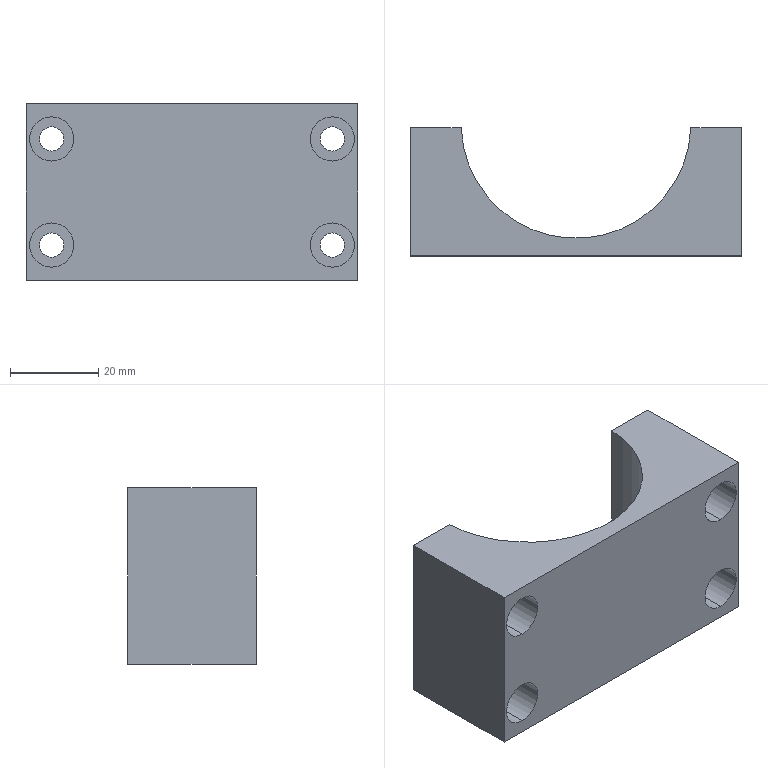Part | SolidWorks | features Extrusion 1, HoleWzd 1, ICE 1, MoveFace 1 | 1 solid | 28 faces | box 75 x 29 x 40 mm | volume 38371 mm3 | cylinder 17 | plane 11 | commonest cylinder face diameters 5.5 x8 10 x8 52 x1
STEP:
#1=CARTESIAN_POINT('',(-31.75,10.,13.));
#2=VERTEX_POINT('',#1);
#3=CARTESIAN_POINT('',(-31.75,10.,3.));
#4=VERTEX_POINT('',#3);
#5=CARTESIAN_POINT('',(-31.75,10.,8.));
#6=DIRECTION('',(0.,-1.,0.));
#7=DIRECTION('',(0.,0.,-1.));
#8=AXIS2_PLACEMENT_3D('',#5,#6,#7);
#9=CIRCLE('',#8,5.);
#10=EDGE_CURVE('',#2,#4,#9,.T.);
#11=ORIENTED_EDGE('',*,*,#10,.F.);
#12=CARTESIAN_POINT('',(-31.75,-15.,13.));
#13=VERTEX_POINT('',#12);
#14=CARTESIAN_POINT('',(-31.75,-15.,13.));
#15=DIRECTION('',(0.,-1.,0.));
#16=VECTOR('',#15,1000.);
#17=LINE('',#14,#16);
#18=EDGE_CURVE('',#2,#13,#17,.T.);
#19=ORIENTED_EDGE('',*,*,#18,.T.);
#20=CARTESIAN_POINT('',(-31.75,-15.,3.));
#21=VERTEX_POINT('',#20);
#22=CARTESIAN_POINT('',(-31.75,-15.,8.));
#23=DIRECTION('',(0.,-1.,0.));
#24=DIRECTION('',(0.,0.,-1.));
#25=AXIS2_PLACEMENT_3D('',#22,#23,#24);
#26=CIRCLE('',#25,5.);
#27=EDGE_CURVE('',#13,#21,#26,.T.);
#28=ORIENTED_EDGE('',*,*,#27,.T.);
#29=CARTESIAN_POINT('',(-31.75,-15.,3.));
#30=DIRECTION('',(0.,-1.,0.));
#31=VECTOR('',#30,1000.);
#32=LINE('',#29,#31);
#33=EDGE_CURVE('',#4,#21,#32,.T.);
#34=ORIENTED_EDGE('',*,*,#33,.F.);
#35=EDGE_LOOP('',(#11,#19,#28,#34));
#36=FACE_OUTER_BOUND('',#35,.T.);
#37=CARTESIAN_POINT('',(-31.75,-15.,8.));
#38=DIRECTION('',(0.,-1.,0.));
#39=DIRECTION('',(0.,0.,-1.));
#40=AXIS2_PLACEMENT_3D('',#37,#38,#39);
#41=CYLINDRICAL_SURFACE('',#40,5.);
#42=ADVANCED_FACE('',(#36),#41,.F.);
#43=CARTESIAN_POINT('',(-31.75,14.,10.75));
#44=VERTEX_POINT('',#43);
#45=CARTESIAN_POINT('',(-31.75,14.,5.25));
#46=VERTEX_POINT('',#45);
#47=CARTESIAN_POINT('',(-31.75,14.,8.));
#48=DIRECTION('',(0.,-1.,0.));
#49=DIRECTION('',(0.,0.,-1.));
#50=AXIS2_PLACEMENT_3D('',#47,#48,#49);
#51=CIRCLE('',#50,2.75);
#52=EDGE_CURVE('',#44,#46,#51,.T.);
#53=ORIENTED_EDGE('',*,*,#52,.F.);
#54=CARTESIAN_POINT('',(-31.75,10.,10.75));
#55=VERTEX_POINT('',#54);
#56=CARTESIAN_POINT('',(-31.75,-15.,10.75));
#57=DIRECTION('',(0.,-1.,0.));
#58=VECTOR('',#57,1000.);
#59=LINE('',#56,#58);
#60=EDGE_CURVE('',#44,#55,#59,.T.);
#61=ORIENTED_EDGE('',*,*,#60,.T.);
#62=CARTESIAN_POINT('',(-31.75,10.,5.25));
#63=VERTEX_POINT('',#62);
#64=CARTESIAN_POINT('',(-31.75,10.,8.));
#65=DIRECTION('',(0.,-1.,0.));
#66=DIRECTION('',(0.,0.,-1.));
#67=AXIS2_PLACEMENT_3D('',#64,#65,#66);
#68=CIRCLE('',#67,2.75);
#69=EDGE_CURVE('',#55,#63,#68,.T.);
#70=ORIENTED_EDGE('',*,*,#69,.T.);
#71=CARTESIAN_POINT('',(-31.75,-15.,5.25));
#72=DIRECTION('',(0.,-1.,0.));
#73=VECTOR('',#72,1000.);
#74=LINE('',#71,#73);
#75=EDGE_CURVE('',#46,#63,#74,.T.);
#76=ORIENTED_EDGE('',*,*,#75,.F.);
#77=EDGE_LOOP('',(#53,#61,#70,#76));
#78=FACE_OUTER_BOUND('',#77,.T.);
#79=CARTESIAN_POINT('',(-31.75,-15.,8.));
#80=DIRECTION('',(0.,-1.,0.));
#81=DIRECTION('',(0.,0.,-1.));
#82=AXIS2_PLACEMENT_3D('',#79,#80,#81);
#83=CYLINDRICAL_SURFACE('',#82,2.75);
#84=ADVANCED_FACE('',(#78),#83,.F.);
#85=CARTESIAN_POINT('',(-31.75,10.,37.));
#86=VERTEX_POINT('',#85);
#87=CARTESIAN_POINT('',(-31.75,10.,27.));
#88=VERTEX_POINT('',#87);
#89=CARTESIAN_POINT('',(-31.75,10.,32.));
#90=DIRECTION('',(0.,-1.,0.));
#91=DIRECTION('',(0.,0.,-1.));
#92=AXIS2_PLACEMENT_3D('',#89,#90,#91);
#93=CIRCLE('',#92,5.);
#94=EDGE_CURVE('',#86,#88,#93,.T.);
#95=ORIENTED_EDGE('',*,*,#94,.F.);
#96=CARTESIAN_POINT('',(-31.75,-15.,37.));
#97=VERTEX_POINT('',#96);
#98=CARTESIAN_POINT('',(-31.75,-15.,37.));
#99=DIRECTION('',(0.,-1.,0.));
#100=VECTOR('',#99,1000.);
#101=LINE('',#98,#100);
#102=EDGE_CURVE('',#86,#97,#101,.T.);
#103=ORIENTED_EDGE('',*,*,#102,.T.);
#104=CARTESIAN_POINT('',(-31.75,-15.,27.));
#105=VERTEX_POINT('',#104);
#106=CARTESIAN_POINT('',(-31.75,-15.,32.));
#107=DIRECTION('',(0.,-1.,0.));
#108=DIRECTION('',(0.,0.,-1.));
#109=AXIS2_PLACEMENT_3D('',#106,#107,#108);
#110=CIRCLE('',#109,5.);
#111=EDGE_CURVE('',#97,#105,#110,.T.);
#112=ORIENTED_EDGE('',*,*,#111,.T.);
#113=CARTESIAN_POINT('',(-31.75,-15.,27.));
#114=DIRECTION('',(0.,-1.,0.));
#115=VECTOR('',#114,1000.);
#116=LINE('',#113,#115);
#117=EDGE_CURVE('',#88,#105,#116,.T.);
#118=ORIENTED_EDGE('',*,*,#117,.F.);
#119=EDGE_LOOP('',(#95,#103,#112,#118));
#120=FACE_OUTER_BOUND('',#119,.T.);
#121=CARTESIAN_POINT('',(-31.75,-15.,32.));
#122=DIRECTION('',(0.,-1.,0.));
#123=DIRECTION('',(0.,0.,-1.));
#124=AXIS2_PLACEMENT_3D('',#121,#122,#123);
#125=CYLINDRICAL_SURFACE('',#124,5.);
#126=ADVANCED_FACE('',(#120),#125,.F.);
#127=CARTESIAN_POINT('',(-31.75,14.,34.75));
#128=VERTEX_POINT('',#127);
#129=CARTESIAN_POINT('',(-31.75,14.,29.25));
#130=VERTEX_POINT('',#129);
#131=CARTESIAN_POINT('',(-31.75,14.,32.));
#132=DIRECTION('',(0.,-1.,0.));
#133=DIRECTION('',(0.,0.,-1.));
#134=AXIS2_PLACEMENT_3D('',#131,#132,#133);
#135=CIRCLE('',#134,2.75);
#136=EDGE_CURVE('',#128,#130,#135,.T.);
#137=ORIENTED_EDGE('',*,*,#136,.F.);
#138=CARTESIAN_POINT('',(-31.75,10.,34.75));
#139=VERTEX_POINT('',#138);
#140=CARTESIAN_POINT('',(-31.75,-15.,34.75));
#141=DIRECTION('',(0.,-1.,0.));
#142=VECTOR('',#141,1000.);
#143=LINE('',#140,#142);
#144=EDGE_CURVE('',#128,#139,#143,.T.);
#145=ORIENTED_EDGE('',*,*,#144,.T.);
#146=CARTESIAN_POINT('',(-31.75,10.,29.25));
#147=VERTEX_POINT('',#146);
#148=CARTESIAN_POINT('',(-31.75,10.,32.));
#149=DIRECTION('',(0.,-1.,0.));
#150=DIRECTION('',(0.,0.,-1.));
#151=AXIS2_PLACEMENT_3D('',#148,#149,#150);
#152=CIRCLE('',#151,2.75);
#153=EDGE_CURVE('',#139,#147,#152,.T.);
#154=ORIENTED_EDGE('',*,*,#153,.T.);
#155=CARTESIAN_POINT('',(-31.75,-15.,29.25));
#156=DIRECTION('',(0.,-1.,0.));
#157=VECTOR('',#156,1000.);
#158=LINE('',#155,#157);
#159=EDGE_CURVE('',#130,#147,#158,.T.);
#160=ORIENTED_EDGE('',*,*,#159,.F.);
#161=EDGE_LOOP('',(#137,#145,#154,#160));
#162=FACE_OUTER_BOUND('',#161,.T.);
#163=CARTESIAN_POINT('',(-31.75,-15.,32.));
#164=DIRECTION('',(0.,-1.,0.));
#165=DIRECTION('',(0.,0.,-1.));
#166=AXIS2_PLACEMENT_3D('',#163,#164,#165);
#167=CYLINDRICAL_SURFACE('',#166,2.75);
#168=ADVANCED_FACE('',(#162),#167,.F.);
#169=CARTESIAN_POINT('',(31.75,10.,37.));
#170=VERTEX_POINT('',#169);
#171=CARTESIAN_POINT('',(31.75,10.,27.));
#172=VERTEX_POINT('',#171);
#173=CARTESIAN_POINT('',(31.75,10.,32.));
#174=DIRECTION('',(0.,-1.,0.));
#175=DIRECTION('',(0.,0.,-1.));
#176=AXIS2_PLACEMENT_3D('',#173,#174,#175);
#177=CIRCLE('',#176,5.);
#178=EDGE_CURVE('',#170,#172,#177,.T.);
#179=ORIENTED_EDGE('',*,*,#178,.F.);
#180=CARTESIAN_POINT('',(31.75,-15.,37.));
#181=VERTEX_POINT('',#180);
#182=CARTESIAN_POINT('',(31.75,-15.,37.));
#183=DIRECTION('',(0.,-1.,0.));
#184=VECTOR('',#183,1000.);
#185=LINE('',#182,#184);
#186=EDGE_CURVE('',#170,#181,#185,.T.);
#187=ORIENTED_EDGE('',*,*,#186,.T.);
#188=CARTESIAN_POINT('',(31.75,-15.,27.));
#189=VERTEX_POINT('',#188);
#190=CARTESIAN_POINT('',(31.75,-15.,32.));
#191=DIRECTION('',(0.,-1.,0.));
#192=DIRECTION('',(0.,0.,-1.));
#193=AXIS2_PLACEMENT_3D('',#190,#191,#192);
#194=CIRCLE('',#193,5.);
#195=EDGE_CURVE('',#181,#189,#194,.T.);
#196=ORIENTED_EDGE('',*,*,#195,.T.);
#197=CARTESIAN_POINT('',(31.75,-15.,27.));
#198=DIRECTION('',(0.,-1.,0.));
#199=VECTOR('',#198,1000.);
#200=LINE('',#197,#199);
#201=EDGE_CURVE('',#172,#189,#200,.T.);
#202=ORIENTED_EDGE('',*,*,#201,.F.);
#203=EDGE_LOOP('',(#179,#187,#196,#202));
#204=FACE_OUTER_BOUND('',#203,.T.);
#205=CARTESIAN_POINT('',(31.75,-15.,32.));
#206=DIRECTION('',(0.,-1.,0.));
#207=DIRECTION('',(0.,0.,-1.));
#208=AXIS2_PLACEMENT_3D('',#205,#206,#207);
#209=CYLINDRICAL_SURFACE('',#208,5.);
#210=ADVANCED_FACE('',(#204),#209,.F.);
#211=CARTESIAN_POINT('',(31.75,14.,34.75));
#212=VERTEX_POINT('',#211);
#213=CARTESIAN_POINT('',(31.75,14.,29.25));
#214=VERTEX_POINT('',#213);
#215=CARTESIAN_POINT('',(31.75,14.,32.));
#216=DIRECTION('',(0.,-1.,0.));
#217=DIRECTION('',(0.,0.,-1.));
#218=AXIS2_PLACEMENT_3D('',#215,#216,#217);
#219=CIRCLE('',#218,2.75);
#220=EDGE_CURVE('',#212,#214,#219,.T.);
#221=ORIENTED_EDGE('',*,*,#220,.F.);
#222=CARTESIAN_POINT('',(31.75,10.,34.75));
#223=VERTEX_POINT('',#222);
#224=CARTESIAN_POINT('',(31.75,-15.,34.75));
#225=DIRECTION('',(0.,-1.,0.));
#226=VECTOR('',#225,1000.);
#227=LINE('',#224,#226);
#228=EDGE_CURVE('',#212,#223,#227,.T.);
#229=ORIENTED_EDGE('',*,*,#228,.T.);
#230=CARTESIAN_POINT('',(31.75,10.,29.25));
#231=VERTEX_POINT('',#230);
#232=CARTESIAN_POINT('',(31.75,10.,32.));
#233=DIRECTION('',(0.,-1.,0.));
#234=DIRECTION('',(0.,0.,-1.));
#235=AXIS2_PLACEMENT_3D('',#232,#233,#234);
#236=CIRCLE('',#235,2.75);
#237=EDGE_CURVE('',#223,#231,#236,.T.);
#238=ORIENTED_EDGE('',*,*,#237,.T.);
#239=CARTESIAN_POINT('',(31.75,-15.,29.25));
#240=DIRECTION('',(0.,-1.,0.));
#241=VECTOR('',#240,1000.);
#242=LINE('',#239,#241);
#243=EDGE_CURVE('',#214,#231,#242,.T.);
#244=ORIENTED_EDGE('',*,*,#243,.F.);
#245=EDGE_LOOP('',(#221,#229,#238,#244));
#246=FACE_OUTER_BOUND('',#245,.T.);
#247=CARTESIAN_POINT('',(31.75,-15.,32.));
#248=DIRECTION('',(0.,-1.,0.));
#249=DIRECTION('',(0.,0.,-1.));
#250=AXIS2_PLACEMENT_3D('',#247,#248,#249);
#251=CYLINDRICAL_SURFACE('',#250,2.75);
#252=ADVANCED_FACE('',(#246),#251,.F.);
#253=CARTESIAN_POINT('',(31.75,10.,13.));
#254=VERTEX_POINT('',#253);
#255=CARTESIAN_POINT('',(31.75,10.,3.));
#256=VERTEX_POINT('',#255);
#257=CARTESIAN_POINT('',(31.75,10.,8.));
#258=DIRECTION('',(0.,-1.,0.));
#259=DIRECTION('',(0.,0.,-1.));
#260=AXIS2_PLACEMENT_3D('',#257,#258,#259);
#261=CIRCLE('',#260,5.);
#262=EDGE_CURVE('',#254,#256,#261,.T.);
#263=ORIENTED_EDGE('',*,*,#262,.F.);
#264=CARTESIAN_POINT('',(31.75,-15.,13.));
#265=VERTEX_POINT('',#264);
#266=CARTESIAN_POINT('',(31.75,-15.,13.));
#267=DIRECTION('',(0.,-1.,0.));
#268=VECTOR('',#267,1000.);
#269=LINE('',#266,#268);
#270=EDGE_CURVE('',#254,#265,#269,.T.);
#271=ORIENTED_EDGE('',*,*,#270,.T.);
#272=CARTESIAN_POINT('',(31.75,-15.,3.));
#273=VERTEX_POINT('',#272);
#274=CARTESIAN_POINT('',(31.75,-15.,8.));
#275=DIRECTION('',(0.,-1.,0.));
#276=DIRECTION('',(0.,0.,-1.));
#277=AXIS2_PLACEMENT_3D('',#274,#275,#276);
#278=CIRCLE('',#277,5.);
#279=EDGE_CURVE('',#265,#273,#278,.T.);
#280=ORIENTED_EDGE('',*,*,#279,.T.);
#281=CARTESIAN_POINT('',(31.75,-15.,3.));
#282=DIRECTION('',(0.,-1.,0.));
#283=VECTOR('',#282,1000.);
#284=LINE('',#281,#283);
#285=EDGE_CURVE('',#256,#273,#284,.T.);
#286=ORIENTED_EDGE('',*,*,#285,.F.);
#287=EDGE_LOOP('',(#263,#271,#280,#286));
#288=FACE_OUTER_BOUND('',#287,.T.);
#289=CARTESIAN_POINT('',(31.75,-15.,8.));
#290=DIRECTION('',(0.,-1.,0.));
#291=DIRECTION('',(0.,0.,-1.));
#292=AXIS2_PLACEMENT_3D('',#289,#290,#291);
#293=CYLINDRICAL_SURFACE('',#292,5.);
#294=ADVANCED_FACE('',(#288),#293,.F.);
#295=CARTESIAN_POINT('',(31.75,14.,10.75));
#296=VERTEX_POINT('',#295);
#297=CARTESIAN_POINT('',(31.75,14.,5.25));
#298=VERTEX_POINT('',#297);
#299=CARTESIAN_POINT('',(31.75,14.,8.));
#300=DIRECTION('',(0.,-1.,0.));
#301=DIRECTION('',(0.,0.,-1.));
#302=AXIS2_PLACEMENT_3D('',#299,#300,#301);
#303=CIRCLE('',#302,2.75);
#304=EDGE_CURVE('',#296,#298,#303,.T.);
#305=ORIENTED_EDGE('',*,*,#304,.F.);
#306=CARTESIAN_POINT('',(31.75,10.,10.75));
#307=VERTEX_POINT('',#306);
#308=CARTESIAN_POINT('',(31.75,-15.,10.75));
#309=DIRECTION('',(0.,-1.,0.));
#310=VECTOR('',#309,1000.);
#311=LINE('',#308,#310);
#312=EDGE_CURVE('',#296,#307,#311,.T.);
#313=ORIENTED_EDGE('',*,*,#312,.T.);
#314=CARTESIAN_POINT('',(31.75,10.,5.25));
#315=VERTEX_POINT('',#314);
#316=CARTESIAN_POINT('',(31.75,10.,8.));
#317=DIRECTION('',(0.,-1.,0.));
#318=DIRECTION('',(0.,0.,-1.));
#319=AXIS2_PLACEMENT_3D('',#316,#317,#318);
#320=CIRCLE('',#319,2.75);
#321=EDGE_CURVE('',#307,#315,#320,.T.);
#322=ORIENTED_EDGE('',*,*,#321,.T.);
#323=CARTESIAN_POINT('',(31.75,-15.,5.25));
#324=DIRECTION('',(0.,-1.,0.));
#325=VECTOR('',#324,1000.);
#326=LINE('',#323,#325);
#327=EDGE_CURVE('',#298,#315,#326,.T.);
#328=ORIENTED_EDGE('',*,*,#327,.F.);
#329=EDGE_LOOP('',(#305,#313,#322,#328));
#330=FACE_OUTER_BOUND('',#329,.T.);
#331=CARTESIAN_POINT('',(31.75,-15.,8.));
#332=DIRECTION('',(0.,-1.,0.));
#333=DIRECTION('',(0.,0.,-1.));
#334=AXIS2_PLACEMENT_3D('',#331,#332,#333);
#335=CYLINDRICAL_SURFACE('',#334,2.75);
#336=ADVANCED_FACE('',(#330),#335,.F.);
#337=CARTESIAN_POINT('',(31.75,14.,32.));
#338=DIRECTION('',(0.,-1.,0.));
#339=DIRECTION('',(0.,0.,-1.));
#340=AXIS2_PLACEMENT_3D('',#337,#338,#339);
#341=CIRCLE('',#340,2.75);
#342=EDGE_CURVE('',#214,#212,#341,.T.);
#343=ORIENTED_EDGE('',*,*,#342,.T.);
#344=ORIENTED_EDGE('',*,*,#220,.T.);
#345=EDGE_LOOP('',(#343,#344));
#346=FACE_BOUND('',#345,.T.);
#347=CARTESIAN_POINT('',(31.75,14.,8.));
#348=DIRECTION('',(0.,-1.,0.));
#349=DIRECTION('',(0.,0.,-1.));
#350=AXIS2_PLACEMENT_3D('',#347,#348,#349);
#351=CIRCLE('',#350,2.75);
#352=EDGE_CURVE('',#298,#296,#351,.T.);
#353=ORIENTED_EDGE('',*,*,#352,.T.);
#354=ORIENTED_EDGE('',*,*,#304,.T.);
#355=EDGE_LOOP('',(#353,#354));
#356=FACE_BOUND('',#355,.T.);
#357=CARTESIAN_POINT('',(37.5,14.,0.));
#358=VERTEX_POINT('',#357);
#359=CARTESIAN_POINT('',(25.981,14.,0.));
#360=VERTEX_POINT('',#359);
#361=CARTESIAN_POINT('',(-37.5,14.,0.));
#362=DIRECTION('',(-1.,0.,0.));
#363=VECTOR('',#362,1000.);
#364=LINE('',#361,#363);
#365=EDGE_CURVE('',#358,#360,#364,.T.);
#366=ORIENTED_EDGE('',*,*,#365,.T.);
#367=CARTESIAN_POINT('',(25.981,14.,40.));
#368=VERTEX_POINT('',#367);
#369=CARTESIAN_POINT('',(25.981,14.,0.));
#370=DIRECTION('',(0.,0.,1.));
#371=VECTOR('',#370,1000.);
#372=LINE('',#369,#371);
#373=EDGE_CURVE('',#360,#368,#372,.T.);
#374=ORIENTED_EDGE('',*,*,#373,.T.);
#375=CARTESIAN_POINT('',(37.5,14.,40.));
#376=VERTEX_POINT('',#375);
#377=CARTESIAN_POINT('',(-37.5,14.,40.));
#378=DIRECTION('',(-1.,0.,0.));
#379=VECTOR('',#378,1000.);
#380=LINE('',#377,#379);
#381=EDGE_CURVE('',#376,#368,#380,.T.);
#382=ORIENTED_EDGE('',*,*,#381,.F.);
#383=CARTESIAN_POINT('',(37.5,14.,40.));
#384=DIRECTION('',(0.,0.,-1.));
#385=VECTOR('',#384,1000.);
#386=LINE('',#383,#385);
#387=EDGE_CURVE('',#376,#358,#386,.T.);
#388=ORIENTED_EDGE('',*,*,#387,.T.);
#389=EDGE_LOOP('',(#366,#374,#382,#388));
#390=FACE_OUTER_BOUND('',#389,.T.);
#391=CARTESIAN_POINT('',(-37.5,14.,40.));
#392=DIRECTION('',(0.,-1.,0.));
#393=DIRECTION('',(0.,0.,-1.));
#394=AXIS2_PLACEMENT_3D('',#391,#392,#393);
#395=PLANE('',#394);
#396=ADVANCED_FACE('',(#346,#356,#390),#395,.F.);
#397=CARTESIAN_POINT('',(37.5,-15.,0.));
#398=VERTEX_POINT('',#397);
#399=CARTESIAN_POINT('',(37.5,-15.,0.));
#400=DIRECTION('',(0.,1.,0.));
#401=VECTOR('',#400,1000.);
#402=LINE('',#399,#401);
#403=EDGE_CURVE('',#398,#358,#402,.T.);
#404=ORIENTED_EDGE('',*,*,#403,.T.);
#405=ORIENTED_EDGE('',*,*,#387,.F.);
#406=CARTESIAN_POINT('',(37.5,-15.,40.));
#407=VERTEX_POINT('',#406);
#408=CARTESIAN_POINT('',(37.5,-15.,40.));
#409=DIRECTION('',(0.,1.,0.));
#410=VECTOR('',#409,1000.);
#411=LINE('',#408,#410);
#412=EDGE_CURVE('',#407,#376,#411,.T.);
#413=ORIENTED_EDGE('',*,*,#412,.F.);
#414=CARTESIAN_POINT('',(37.5,-15.,40.));
#415=DIRECTION('',(0.,0.,-1.));
#416=VECTOR('',#415,1000.);
#417=LINE('',#414,#416);
#418=EDGE_CURVE('',#407,#398,#417,.T.);
#419=ORIENTED_EDGE('',*,*,#418,.T.);
#420=EDGE_LOOP('',(#404,#405,#413,#419));
#421=FACE_OUTER_BOUND('',#420,.T.);
#422=CARTESIAN_POINT('',(37.5,-15.,40.));
#423=DIRECTION('',(-1.,0.,0.));
#424=DIRECTION('',(0.,0.,1.));
#425=AXIS2_PLACEMENT_3D('',#422,#423,#424);
#426=PLANE('',#425);
#427=ADVANCED_FACE('',(#421),#426,.F.);
#428=CARTESIAN_POINT('',(-31.75,14.,8.));
#429=DIRECTION('',(0.,-1.,0.));
#430=DIRECTION('',(0.,0.,-1.));
#431=AXIS2_PLACEMENT_3D('',#428,#429,#430);
#432=CIRCLE('',#431,2.75);
#433=EDGE_CURVE('',#46,#44,#432,.T.);
#434=ORIENTED_EDGE('',*,*,#433,.T.);
#435=ORIENTED_EDGE('',*,*,#52,.T.);
#436=EDGE_LOOP('',(#434,#435));
#437=FACE_BOUND('',#436,.T.);
#438=CARTESIAN_POINT('',(-31.75,14.,32.));
#439=DIRECTION('',(0.,-1.,0.));
#440=DIRECTION('',(0.,0.,-1.));
#441=AXIS2_PLACEMENT_3D('',#438,#439,#440);
#442=CIRCLE('',#441,2.75);
#443=EDGE_CURVE('',#130,#128,#442,.T.);
#444=ORIENTED_EDGE('',*,*,#443,.T.);
#445=ORIENTED_EDGE('',*,*,#136,.T.);
#446=EDGE_LOOP('',(#444,#445));
#447=FACE_BOUND('',#446,.T.);
#448=CARTESIAN_POINT('',(-25.981,14.,40.));
#449=VERTEX_POINT('',#448);
#450=CARTESIAN_POINT('',(-37.5,14.,40.));
#451=VERTEX_POINT('',#450);
#452=CARTESIAN_POINT('',(-37.5,14.,40.));
#453=DIRECTION('',(-1.,0.,0.));
#454=VECTOR('',#453,1000.);
#455=LINE('',#452,#454);
#456=EDGE_CURVE('',#449,#451,#455,.T.);
#457=ORIENTED_EDGE('',*,*,#456,.F.);
#458=CARTESIAN_POINT('',(-25.981,14.,0.));
#459=VERTEX_POINT('',#458);
#460=CARTESIAN_POINT('',(-25.981,14.,40.));
#461=DIRECTION('',(0.,0.,-1.));
#462=VECTOR('',#461,1000.);
#463=LINE('',#460,#462);
#464=EDGE_CURVE('',#449,#459,#463,.T.);
#465=ORIENTED_EDGE('',*,*,#464,.T.);
#466=CARTESIAN_POINT('',(-37.5,14.,0.));
#467=VERTEX_POINT('',#466);
#468=CARTESIAN_POINT('',(-37.5,14.,0.));
#469=DIRECTION('',(-1.,0.,0.));
#470=VECTOR('',#469,1000.);
#471=LINE('',#468,#470);
#472=EDGE_CURVE('',#459,#467,#471,.T.);
#473=ORIENTED_EDGE('',*,*,#472,.T.);
#474=CARTESIAN_POINT('',(-37.5,14.,40.));
#475=DIRECTION('',(0.,0.,-1.));
#476=VECTOR('',#475,1000.);
#477=LINE('',#474,#476);
#478=EDGE_CURVE('',#451,#467,#477,.T.);
#479=ORIENTED_EDGE('',*,*,#478,.F.);
#480=EDGE_LOOP('',(#457,#465,#473,#479));
#481=FACE_OUTER_BOUND('',#480,.T.);
#482=CARTESIAN_POINT('',(-37.5,14.,40.));
#483=DIRECTION('',(0.,-1.,0.));
#484=DIRECTION('',(0.,0.,-1.));
#485=AXIS2_PLACEMENT_3D('',#482,#483,#484);
#486=PLANE('',#485);
#487=ADVANCED_FACE('',(#437,#447,#481),#486,.F.);
#488=CARTESIAN_POINT('',(-37.5,-15.,0.));
#489=VERTEX_POINT('',#488);
#490=CARTESIAN_POINT('',(-37.5,-15.,0.));
#491=DIRECTION('',(0.,-1.,0.));
#492=VECTOR('',#491,1000.);
#493=LINE('',#490,#492);
#494=EDGE_CURVE('',#467,#489,#493,.T.);
#495=ORIENTED_EDGE('',*,*,#494,.T.);
#496=CARTESIAN_POINT('',(-37.5,-15.,40.));
#497=VERTEX_POINT('',#496);
#498=CARTESIAN_POINT('',(-37.5,-15.,40.));
#499=DIRECTION('',(0.,0.,-1.));
#500=VECTOR('',#499,1000.);
#501=LINE('',#498,#500);
#502=EDGE_CURVE('',#497,#489,#501,.T.);
#503=ORIENTED_EDGE('',*,*,#502,.F.);
#504=CARTESIAN_POINT('',(-37.5,-15.,40.));
#505=DIRECTION('',(0.,-1.,0.));
#506=VECTOR('',#505,1000.);
#507=LINE('',#504,#506);
#508=EDGE_CURVE('',#451,#497,#507,.T.);
#509=ORIENTED_EDGE('',*,*,#508,.F.);
#510=ORIENTED_EDGE('',*,*,#478,.T.);
#511=EDGE_LOOP('',(#495,#503,#509,#510));
#512=FACE_OUTER_BOUND('',#511,.T.);
#513=CARTESIAN_POINT('',(-37.5,-15.,40.));
#514=DIRECTION('',(1.,0.,0.));
#515=DIRECTION('',(0.,0.,-1.));
#516=AXIS2_PLACEMENT_3D('',#513,#514,#515);
#517=PLANE('',#516);
#518=ADVANCED_FACE('',(#512),#517,.F.);
#519=CARTESIAN_POINT('',(-31.75,-15.,8.));
#520=DIRECTION('',(0.,-1.,0.));
#521=DIRECTION('',(0.,0.,-1.));
#522=AXIS2_PLACEMENT_3D('',#519,#520,#521);
#523=CIRCLE('',#522,5.);
#524=EDGE_CURVE('',#21,#13,#523,.T.);
#525=ORIENTED_EDGE('',*,*,#524,.F.);
#526=ORIENTED_EDGE('',*,*,#27,.F.);
#527=EDGE_LOOP('',(#525,#526));
#528=FACE_BOUND('',#527,.T.);
#529=CARTESIAN_POINT('',(-31.75,-15.,32.));
#530=DIRECTION('',(0.,-1.,0.));
#531=DIRECTION('',(0.,0.,-1.));
#532=AXIS2_PLACEMENT_3D('',#529,#530,#531);
#533=CIRCLE('',#532,5.);
#534=EDGE_CURVE('',#105,#97,#533,.T.);
#535=ORIENTED_EDGE('',*,*,#534,.F.);
#536=ORIENTED_EDGE('',*,*,#111,.F.);
#537=EDGE_LOOP('',(#535,#536));
#538=FACE_BOUND('',#537,.T.);
#539=CARTESIAN_POINT('',(31.75,-15.,32.));
#540=DIRECTION('',(0.,-1.,0.));
#541=DIRECTION('',(0.,0.,-1.));
#542=AXIS2_PLACEMENT_3D('',#539,#540,#541);
#543=CIRCLE('',#542,5.);
#544=EDGE_CURVE('',#189,#181,#543,.T.);
#545=ORIENTED_EDGE('',*,*,#544,.F.);
#546=ORIENTED_EDGE('',*,*,#195,.F.);
#547=EDGE_LOOP('',(#545,#546));
#548=FACE_BOUND('',#547,.T.);
#549=CARTESIAN_POINT('',(31.75,-15.,8.));
#550=DIRECTION('',(0.,-1.,0.));
#551=DIRECTION('',(0.,0.,-1.));
#552=AXIS2_PLACEMENT_3D('',#549,#550,#551);
#553=CIRCLE('',#552,5.);
#554=EDGE_CURVE('',#273,#265,#553,.T.);
#555=ORIENTED_EDGE('',*,*,#554,.F.);
#556=ORIENTED_EDGE('',*,*,#279,.F.);
#557=EDGE_LOOP('',(#555,#556));
#558=FACE_BOUND('',#557,.T.);
#559=CARTESIAN_POINT('',(-37.5,-15.,0.));
#560=DIRECTION('',(1.,0.,0.));
#561=VECTOR('',#560,1000.);
#562=LINE('',#559,#561);
#563=EDGE_CURVE('',#489,#398,#562,.T.);
#564=ORIENTED_EDGE('',*,*,#563,.T.);
#565=ORIENTED_EDGE('',*,*,#418,.F.);
#566=CARTESIAN_POINT('',(-37.5,-15.,40.));
#567=DIRECTION('',(1.,0.,0.));
#568=VECTOR('',#567,1000.);
#569=LINE('',#566,#568);
#570=EDGE_CURVE('',#497,#407,#569,.T.);
#571=ORIENTED_EDGE('',*,*,#570,.F.);
#572=ORIENTED_EDGE('',*,*,#502,.T.);
#573=EDGE_LOOP('',(#564,#565,#571,#572));
#574=FACE_OUTER_BOUND('',#573,.T.);
#575=CARTESIAN_POINT('',(-37.5,-15.,40.));
#576=DIRECTION('',(0.,1.,0.));
#577=DIRECTION('',(0.,0.,1.));
#578=AXIS2_PLACEMENT_3D('',#575,#576,#577);
#579=PLANE('',#578);
#580=ADVANCED_FACE('',(#528,#538,#548,#558,#574),#579,.F.);
#581=ORIENTED_EDGE('',*,*,#381,.T.);
#582=CARTESIAN_POINT('',(0.,15.,40.));
#583=DIRECTION('',(0.,0.,1.));
#584=DIRECTION('',(1.,0.,0.));
#585=AXIS2_PLACEMENT_3D('',#582,#583,#584);
#586=CIRCLE('',#585,26.);
#587=EDGE_CURVE('',#449,#368,#586,.T.);
#588=ORIENTED_EDGE('',*,*,#587,.F.);
#589=ORIENTED_EDGE('',*,*,#456,.T.);
#590=ORIENTED_EDGE('',*,*,#508,.T.);
#591=ORIENTED_EDGE('',*,*,#570,.T.);
#592=ORIENTED_EDGE('',*,*,#412,.T.);
#593=EDGE_LOOP('',(#581,#588,#589,#590,#591,#592));
#594=FACE_OUTER_BOUND('',#593,.T.);
#595=CARTESIAN_POINT('',(0.,0.,40.));
#596=DIRECTION('',(0.,0.,-1.));
#597=DIRECTION('',(-1.,0.,0.));
#598=AXIS2_PLACEMENT_3D('',#595,#596,#597);
#599=PLANE('',#598);
#600=ADVANCED_FACE('',(#594),#599,.F.);
#601=CARTESIAN_POINT('',(0.,15.,0.));
#602=DIRECTION('',(0.,0.,-1.));
#603=DIRECTION('',(-1.,0.,0.));
#604=AXIS2_PLACEMENT_3D('',#601,#602,#603);
#605=CIRCLE('',#604,26.);
#606=EDGE_CURVE('',#360,#459,#605,.T.);
#607=ORIENTED_EDGE('',*,*,#606,.F.);
#608=ORIENTED_EDGE('',*,*,#365,.F.);
#609=ORIENTED_EDGE('',*,*,#403,.F.);
#610=ORIENTED_EDGE('',*,*,#563,.F.);
#611=ORIENTED_EDGE('',*,*,#494,.F.);
#612=ORIENTED_EDGE('',*,*,#472,.F.);
#613=EDGE_LOOP('',(#607,#608,#609,#610,#611,#612));
#614=FACE_OUTER_BOUND('',#613,.T.);
#615=CARTESIAN_POINT('',(0.,0.,0.));
#616=DIRECTION('',(0.,0.,-1.));
#617=DIRECTION('',(-1.,0.,0.));
#618=AXIS2_PLACEMENT_3D('',#615,#616,#617);
#619=PLANE('',#618);
#620=ADVANCED_FACE('',(#614),#619,.T.);
#621=ORIENTED_EDGE('',*,*,#606,.T.);
#622=ORIENTED_EDGE('',*,*,#464,.F.);
#623=ORIENTED_EDGE('',*,*,#587,.T.);
#624=ORIENTED_EDGE('',*,*,#373,.F.);
#625=EDGE_LOOP('',(#621,#622,#623,#624));
#626=FACE_OUTER_BOUND('',#625,.T.);
#627=CARTESIAN_POINT('',(0.,15.,0.));
#628=DIRECTION('',(0.,0.,1.));
#629=DIRECTION('',(1.,0.,0.));
#630=AXIS2_PLACEMENT_3D('',#627,#628,#629);
#631=CYLINDRICAL_SURFACE('',#630,26.);
#632=ADVANCED_FACE('',(#626),#631,.F.);
#633=ORIENTED_EDGE('',*,*,#312,.F.);
#634=ORIENTED_EDGE('',*,*,#352,.F.);
#635=ORIENTED_EDGE('',*,*,#327,.T.);
#636=CARTESIAN_POINT('',(31.75,10.,8.));
#637=DIRECTION('',(0.,-1.,0.));
#638=DIRECTION('',(0.,0.,-1.));
#639=AXIS2_PLACEMENT_3D('',#636,#637,#638);
#640=CIRCLE('',#639,2.75);
#641=EDGE_CURVE('',#315,#307,#640,.T.);
#642=ORIENTED_EDGE('',*,*,#641,.T.);
#643=EDGE_LOOP('',(#633,#634,#635,#642));
#644=FACE_OUTER_BOUND('',#643,.T.);
#645=CARTESIAN_POINT('',(31.75,-15.,8.));
#646=DIRECTION('',(0.,-1.,0.));
#647=DIRECTION('',(0.,0.,-1.));
#648=AXIS2_PLACEMENT_3D('',#645,#646,#647);
#649=CYLINDRICAL_SURFACE('',#648,2.75);
#650=ADVANCED_FACE('',(#644),#649,.F.);
#651=ORIENTED_EDGE('',*,*,#641,.F.);
#652=ORIENTED_EDGE('',*,*,#321,.F.);
#653=EDGE_LOOP('',(#651,#652));
#654=FACE_BOUND('',#653,.T.);
#655=CARTESIAN_POINT('',(31.75,10.,8.));
#656=DIRECTION('',(0.,-1.,0.));
#657=DIRECTION('',(0.,0.,-1.));
#658=AXIS2_PLACEMENT_3D('',#655,#656,#657);
#659=CIRCLE('',#658,5.);
#660=EDGE_CURVE('',#256,#254,#659,.T.);
#661=ORIENTED_EDGE('',*,*,#660,.T.);
#662=ORIENTED_EDGE('',*,*,#262,.T.);
#663=EDGE_LOOP('',(#661,#662));
#664=FACE_OUTER_BOUND('',#663,.T.);
#665=CARTESIAN_POINT('',(34.5,10.,8.));
#666=DIRECTION('',(0.,1.,0.));
#667=DIRECTION('',(0.,0.,1.));
#668=AXIS2_PLACEMENT_3D('',#665,#666,#667);
#669=PLANE('',#668);
#670=ADVANCED_FACE('',(#654,#664),#669,.F.);
#671=ORIENTED_EDGE('',*,*,#270,.F.);
#672=ORIENTED_EDGE('',*,*,#660,.F.);
#673=ORIENTED_EDGE('',*,*,#285,.T.);
#674=ORIENTED_EDGE('',*,*,#554,.T.);
#675=EDGE_LOOP('',(#671,#672,#673,#674));
#676=FACE_OUTER_BOUND('',#675,.T.);
#677=CARTESIAN_POINT('',(31.75,-15.,8.));
#678=DIRECTION('',(0.,-1.,0.));
#679=DIRECTION('',(0.,0.,-1.));
#680=AXIS2_PLACEMENT_3D('',#677,#678,#679);
#681=CYLINDRICAL_SURFACE('',#680,5.);
#682=ADVANCED_FACE('',(#676),#681,.F.);
#683=ORIENTED_EDGE('',*,*,#228,.F.);
#684=ORIENTED_EDGE('',*,*,#342,.F.);
#685=ORIENTED_EDGE('',*,*,#243,.T.);
#686=CARTESIAN_POINT('',(31.75,10.,32.));
#687=DIRECTION('',(0.,-1.,0.));
#688=DIRECTION('',(0.,0.,-1.));
#689=AXIS2_PLACEMENT_3D('',#686,#687,#688);
#690=CIRCLE('',#689,2.75);
#691=EDGE_CURVE('',#231,#223,#690,.T.);
#692=ORIENTED_EDGE('',*,*,#691,.T.);
#693=EDGE_LOOP('',(#683,#684,#685,#692));
#694=FACE_OUTER_BOUND('',#693,.T.);
#695=CARTESIAN_POINT('',(31.75,-15.,32.));
#696=DIRECTION('',(0.,-1.,0.));
#697=DIRECTION('',(0.,0.,-1.));
#698=AXIS2_PLACEMENT_3D('',#695,#696,#697);
#699=CYLINDRICAL_SURFACE('',#698,2.75);
#700=ADVANCED_FACE('',(#694),#699,.F.);
#701=ORIENTED_EDGE('',*,*,#691,.F.);
#702=ORIENTED_EDGE('',*,*,#237,.F.);
#703=EDGE_LOOP('',(#701,#702));
#704=FACE_BOUND('',#703,.T.);
#705=CARTESIAN_POINT('',(31.75,10.,32.));
#706=DIRECTION('',(0.,-1.,0.));
#707=DIRECTION('',(0.,0.,-1.));
#708=AXIS2_PLACEMENT_3D('',#705,#706,#707);
#709=CIRCLE('',#708,5.);
#710=EDGE_CURVE('',#172,#170,#709,.T.);
#711=ORIENTED_EDGE('',*,*,#710,.T.);
#712=ORIENTED_EDGE('',*,*,#178,.T.);
#713=EDGE_LOOP('',(#711,#712));
#714=FACE_OUTER_BOUND('',#713,.T.);
#715=CARTESIAN_POINT('',(34.5,10.,32.));
#716=DIRECTION('',(0.,1.,0.));
#717=DIRECTION('',(0.,0.,1.));
#718=AXIS2_PLACEMENT_3D('',#715,#716,#717);
#719=PLANE('',#718);
#720=ADVANCED_FACE('',(#704,#714),#719,.F.);
#721=ORIENTED_EDGE('',*,*,#186,.F.);
#722=ORIENTED_EDGE('',*,*,#710,.F.);
#723=ORIENTED_EDGE('',*,*,#201,.T.);
#724=ORIENTED_EDGE('',*,*,#544,.T.);
#725=EDGE_LOOP('',(#721,#722,#723,#724));
#726=FACE_OUTER_BOUND('',#725,.T.);
#727=CARTESIAN_POINT('',(31.75,-15.,32.));
#728=DIRECTION('',(0.,-1.,0.));
#729=DIRECTION('',(0.,0.,-1.));
#730=AXIS2_PLACEMENT_3D('',#727,#728,#729);
#731=CYLINDRICAL_SURFACE('',#730,5.);
#732=ADVANCED_FACE('',(#726),#731,.F.);
#733=ORIENTED_EDGE('',*,*,#144,.F.);
#734=ORIENTED_EDGE('',*,*,#443,.F.);
#735=ORIENTED_EDGE('',*,*,#159,.T.);
#736=CARTESIAN_POINT('',(-31.75,10.,32.));
#737=DIRECTION('',(0.,-1.,0.));
#738=DIRECTION('',(0.,0.,-1.));
#739=AXIS2_PLACEMENT_3D('',#736,#737,#738);
#740=CIRCLE('',#739,2.75);
#741=EDGE_CURVE('',#147,#139,#740,.T.);
#742=ORIENTED_EDGE('',*,*,#741,.T.);
#743=EDGE_LOOP('',(#733,#734,#735,#742));
#744=FACE_OUTER_BOUND('',#743,.T.);
#745=CARTESIAN_POINT('',(-31.75,-15.,32.));
#746=DIRECTION('',(0.,-1.,0.));
#747=DIRECTION('',(0.,0.,-1.));
#748=AXIS2_PLACEMENT_3D('',#745,#746,#747);
#749=CYLINDRICAL_SURFACE('',#748,2.75);
#750=ADVANCED_FACE('',(#744),#749,.F.);
#751=ORIENTED_EDGE('',*,*,#741,.F.);
#752=ORIENTED_EDGE('',*,*,#153,.F.);
#753=EDGE_LOOP('',(#751,#752));
#754=FACE_BOUND('',#753,.T.);
#755=CARTESIAN_POINT('',(-31.75,10.,32.));
#756=DIRECTION('',(0.,-1.,0.));
#757=DIRECTION('',(0.,0.,-1.));
#758=AXIS2_PLACEMENT_3D('',#755,#756,#757);
#759=CIRCLE('',#758,5.);
#760=EDGE_CURVE('',#88,#86,#759,.T.);
#761=ORIENTED_EDGE('',*,*,#760,.T.);
#762=ORIENTED_EDGE('',*,*,#94,.T.);
#763=EDGE_LOOP('',(#761,#762));
#764=FACE_OUTER_BOUND('',#763,.T.);
#765=CARTESIAN_POINT('',(-29.,10.,32.));
#766=DIRECTION('',(0.,1.,0.));
#767=DIRECTION('',(0.,0.,1.));
#768=AXIS2_PLACEMENT_3D('',#765,#766,#767);
#769=PLANE('',#768);
#770=ADVANCED_FACE('',(#754,#764),#769,.F.);
#771=ORIENTED_EDGE('',*,*,#102,.F.);
#772=ORIENTED_EDGE('',*,*,#760,.F.);
#773=ORIENTED_EDGE('',*,*,#117,.T.);
#774=ORIENTED_EDGE('',*,*,#534,.T.);
#775=EDGE_LOOP('',(#771,#772,#773,#774));
#776=FACE_OUTER_BOUND('',#775,.T.);
#777=CARTESIAN_POINT('',(-31.75,-15.,32.));
#778=DIRECTION('',(0.,-1.,0.));
#779=DIRECTION('',(0.,0.,-1.));
#780=AXIS2_PLACEMENT_3D('',#777,#778,#779);
#781=CYLINDRICAL_SURFACE('',#780,5.);
#782=ADVANCED_FACE('',(#776),#781,.F.);
#783=ORIENTED_EDGE('',*,*,#60,.F.);
#784=ORIENTED_EDGE('',*,*,#433,.F.);
#785=ORIENTED_EDGE('',*,*,#75,.T.);
#786=CARTESIAN_POINT('',(-31.75,10.,8.));
#787=DIRECTION('',(0.,-1.,0.));
#788=DIRECTION('',(0.,0.,-1.));
#789=AXIS2_PLACEMENT_3D('',#786,#787,#788);
#790=CIRCLE('',#789,2.75);
#791=EDGE_CURVE('',#63,#55,#790,.T.);
#792=ORIENTED_EDGE('',*,*,#791,.T.);
#793=EDGE_LOOP('',(#783,#784,#785,#792));
#794=FACE_OUTER_BOUND('',#793,.T.);
#795=CARTESIAN_POINT('',(-31.75,-15.,8.));
#796=DIRECTION('',(0.,-1.,0.));
#797=DIRECTION('',(0.,0.,-1.));
#798=AXIS2_PLACEMENT_3D('',#795,#796,#797);
#799=CYLINDRICAL_SURFACE('',#798,2.75);
#800=ADVANCED_FACE('',(#794),#799,.F.);
#801=ORIENTED_EDGE('',*,*,#791,.F.);
#802=ORIENTED_EDGE('',*,*,#69,.F.);
#803=EDGE_LOOP('',(#801,#802));
#804=FACE_BOUND('',#803,.T.);
#805=CARTESIAN_POINT('',(-31.75,10.,8.));
#806=DIRECTION('',(0.,-1.,0.));
#807=DIRECTION('',(0.,0.,-1.));
#808=AXIS2_PLACEMENT_3D('',#805,#806,#807);
#809=CIRCLE('',#808,5.);
#810=EDGE_CURVE('',#4,#2,#809,.T.);
#811=ORIENTED_EDGE('',*,*,#810,.T.);
#812=ORIENTED_EDGE('',*,*,#10,.T.);
#813=EDGE_LOOP('',(#811,#812));
#814=FACE_OUTER_BOUND('',#813,.T.);
#815=CARTESIAN_POINT('',(-29.,10.,8.));
#816=DIRECTION('',(0.,1.,0.));
#817=DIRECTION('',(0.,0.,1.));
#818=AXIS2_PLACEMENT_3D('',#815,#816,#817);
#819=PLANE('',#818);
#820=ADVANCED_FACE('',(#804,#814),#819,.F.);
#821=ORIENTED_EDGE('',*,*,#18,.F.);
#822=ORIENTED_EDGE('',*,*,#810,.F.);
#823=ORIENTED_EDGE('',*,*,#33,.T.);
#824=ORIENTED_EDGE('',*,*,#524,.T.);
#825=EDGE_LOOP('',(#821,#822,#823,#824));
#826=FACE_OUTER_BOUND('',#825,.T.);
#827=CARTESIAN_POINT('',(-31.75,-15.,8.));
#828=DIRECTION('',(0.,-1.,0.));
#829=DIRECTION('',(0.,0.,-1.));
#830=AXIS2_PLACEMENT_3D('',#827,#828,#829);
#831=CYLINDRICAL_SURFACE('',#830,5.);
#832=ADVANCED_FACE('',(#826),#831,.F.);
#833=CLOSED_SHELL('',(#42,#84,#126,#168,#210,#252,#294,#336,#396,#427,#487,#518,#580,#600,#620,#632,#650,#670,#682,#700,#720,#732,#750,#770,#782,#800,#820,#832));
#834=MANIFOLD_SOLID_BREP('',#833);
#835=CARTESIAN_POINT('',(0.,0.,0.));
#836=DIRECTION('',(0.,0.,1.));
#837=DIRECTION('',(1.,0.,0.));
#838=AXIS2_PLACEMENT_3D('',#835,#836,#837);
#839=(LENGTH_UNIT()NAMED_UNIT(*)SI_UNIT(.MILLI.,.METRE.));
#840=UNCERTAINTY_MEASURE_WITH_UNIT(LENGTH_MEASURE(0.00001),#839,'','');
#841=(NAMED_UNIT(*)PLANE_ANGLE_UNIT()SI_UNIT($,.RADIAN.));
#842=(NAMED_UNIT(*)SI_UNIT($,.STERADIAN.)SOLID_ANGLE_UNIT());
#843=(GEOMETRIC_REPRESENTATION_CONTEXT(3)GLOBAL_UNCERTAINTY_ASSIGNED_CONTEXT((#840))GLOBAL_UNIT_ASSIGNED_CONTEXT((#839,#841,#842))REPRESENTATION_CONTEXT('',''));
#844=ADVANCED_BREP_SHAPE_REPRESENTATION('',(#834,#838),#843);